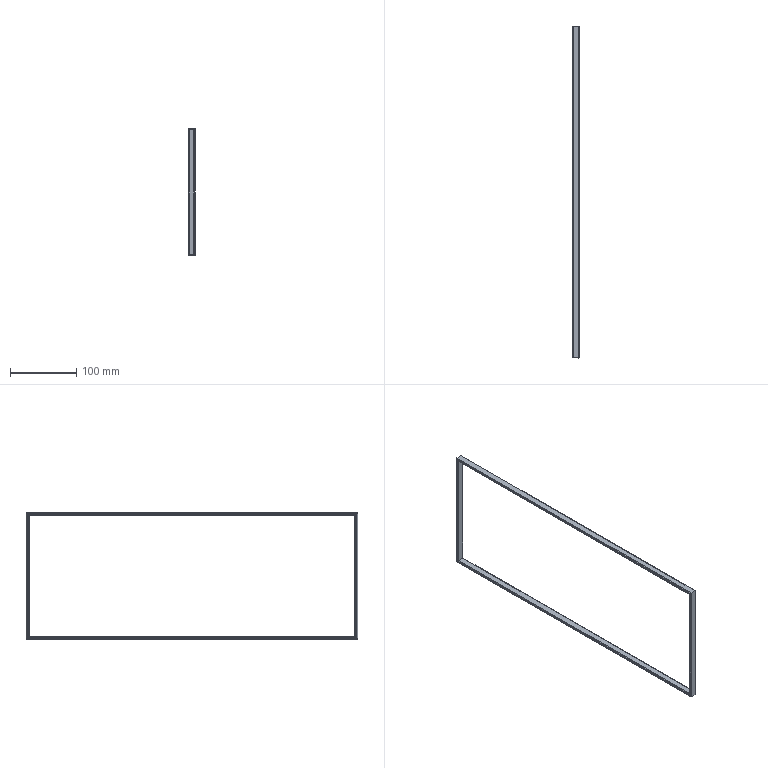Part | STEP file | RJWD-DY-0102_X2_5DE667DC95E8_12 | 1 solid | 36 faces | box 10 x 501.004 x 192.504 mm | volume 49501 mm3 | plane 20 | cylinder 16 | commonest cylinder face diameters 2 x16